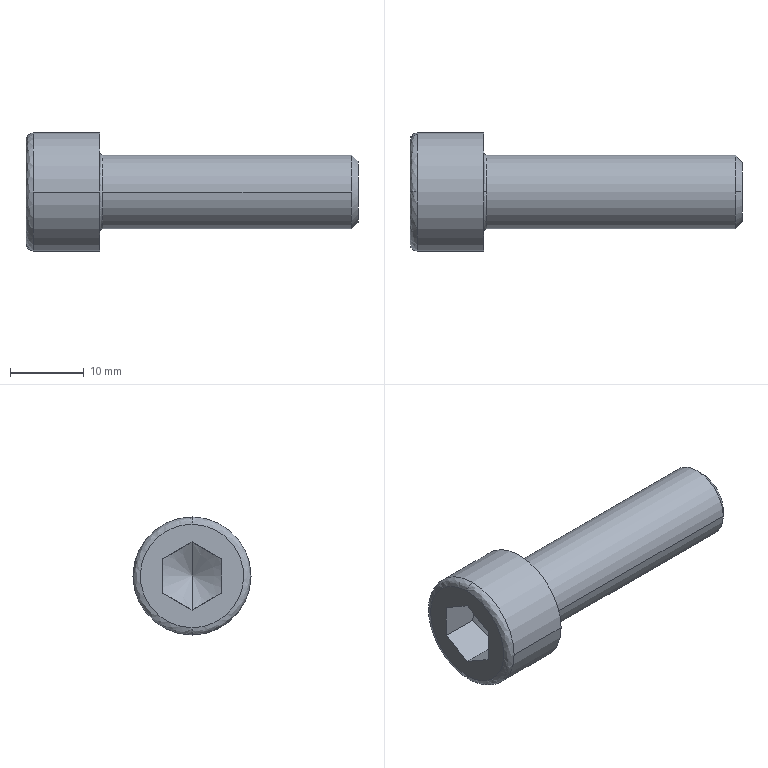Part | STEP file | Broached Socket Head Cap Screw - Metric M10x1.5 x 35 | 1 solid | 21 faces | box 45 x 16 x 16 mm | volume 4403 mm3 | plane 9 | spline 4 | cylinder 4 | cone 4 | commonest cylinder face diameters 10 x2 16 x2